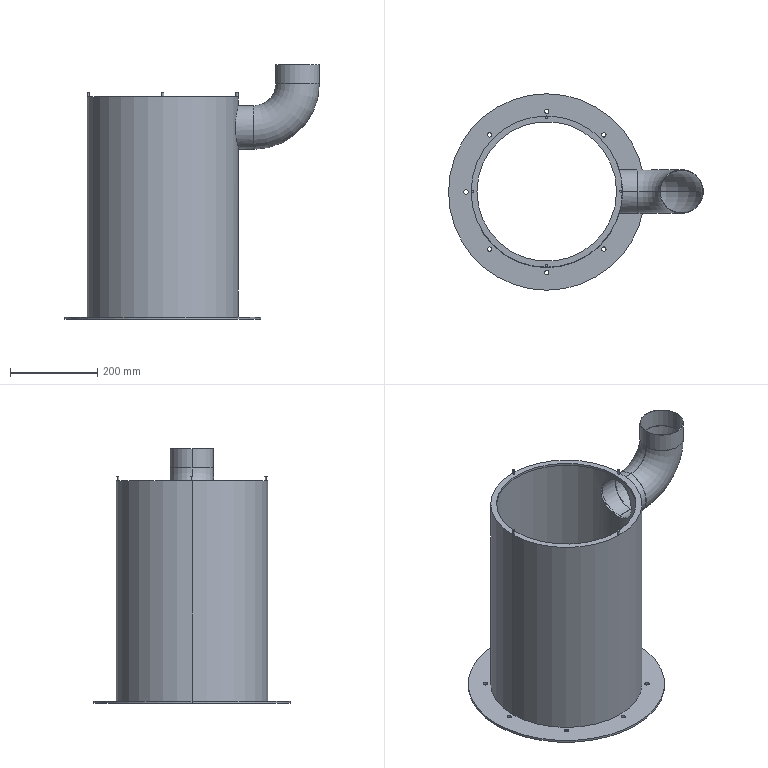Part | SolidWorks | features ICE 5, Cut 2, RefAxis 1, Sweep 1 | 1 solid | 53 faces | box 583.992 x 450 x 583.584 mm | volume 3138291 mm3 | cylinder 40 | plane 9 | torus 4 | commonest cylinder face diameters 10 x16 5 x8 98 x4 100 x4 320 x2 336.734 x2